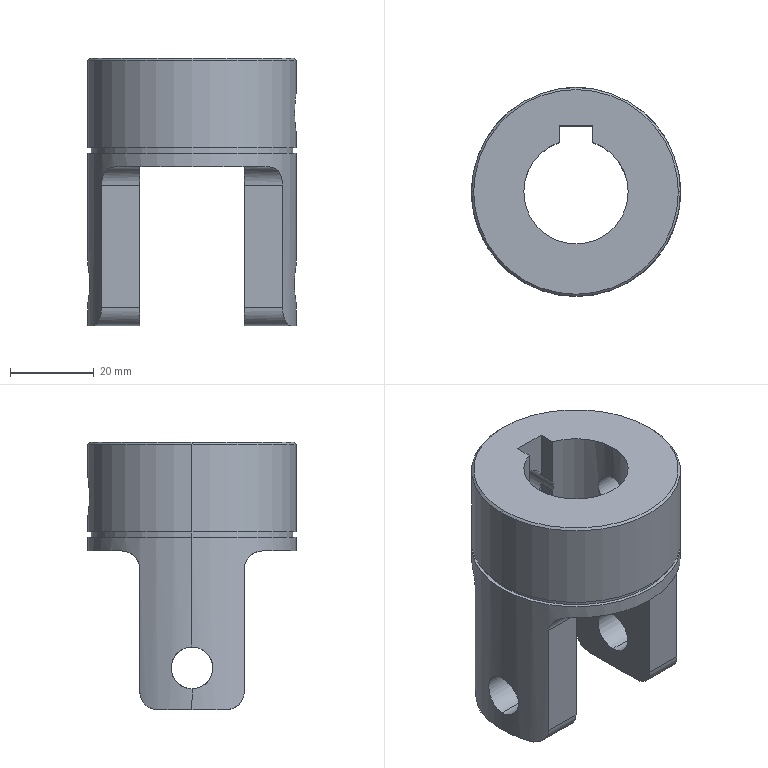Part | SolidWorks | features RefAxis 6, ICE 4, 3DProfileFeature 2, RevCut 2, LockFeature 1, Revolution 1 | 1 solid | 50 faces | box 50 x 50 x 64 mm | volume 55881 mm3 | cylinder 25 | plane 19 | cone 6 | commonest cylinder face diameters 8.667 x8 8.376 x4 10 x4 50 x4 25 x3 48.267 x2